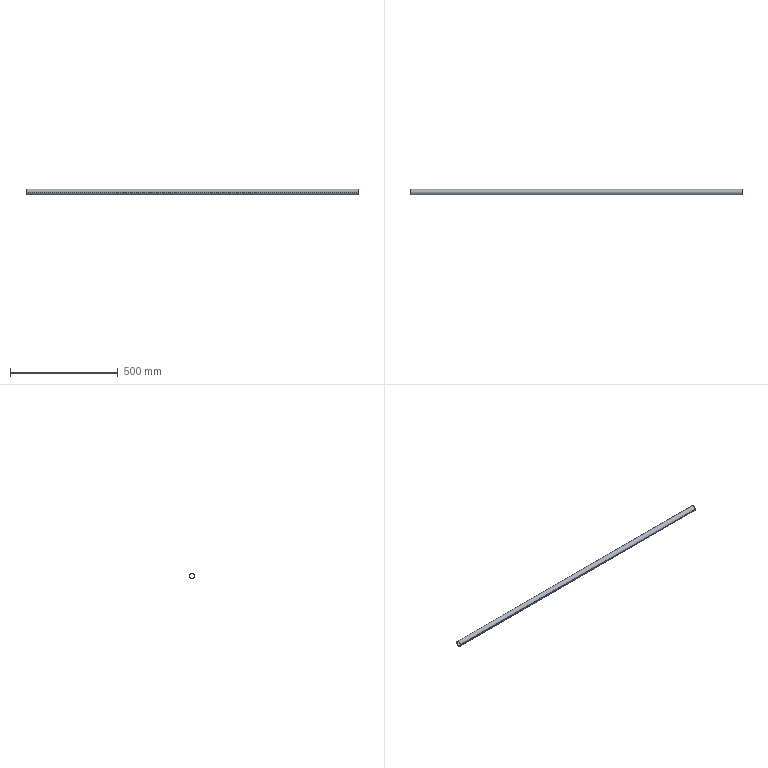Part | STEP file | E3-电柜护栏6栏杆_Default<As Machined> | 1 solid | 6 faces | box 1540 x 25 x 25 mm | volume 170541 mm3 | cylinder 4 | plane 2 | commonest cylinder face diameters 22 x2 25 x2
STEP:
#1=CARTESIAN_POINT('',(0.,0.,0.));
#2=DIRECTION('',(0.,0.,1.));
#3=DIRECTION('',(1.,0.,0.));
#4=AXIS2_PLACEMENT_3D('',#1,#2,#3);
#5=CARTESIAN_POINT('',(770.,-12.5,0.));
#6=VERTEX_POINT('',#5);
#7=CARTESIAN_POINT('',(770.,12.5,0.));
#8=VERTEX_POINT('',#7);
#9=CARTESIAN_POINT('',(770.,0.,0.));
#10=DIRECTION('',(-1.,0.,0.));
#11=DIRECTION('',(0.,1.,0.));
#12=AXIS2_PLACEMENT_3D('',#9,#10,#11);
#13=CIRCLE('',#12,12.5);
#14=CARTESIAN_POINT('',(770.,0.,0.));
#15=DIRECTION('',(-1.,0.,0.));
#16=DIRECTION('',(0.,-1.,0.));
#17=AXIS2_PLACEMENT_3D('',#14,#15,#16);
#18=CYLINDRICAL_SURFACE('',#17,12.5);
#19=CARTESIAN_POINT('',(-3.142,0.));
#20=DIRECTION('',(1.,0.));
#21=VECTOR('',#20,1.);
#22=LINE('',#19,#21);
#23=(GEOMETRIC_REPRESENTATION_CONTEXT(2)PARAMETRIC_REPRESENTATION_CONTEXT()REPRESENTATION_CONTEXT('',''));
#24=DEFINITIONAL_REPRESENTATION('',(#22),#23);
#25=PCURVE('',#18,#24);
#26=CARTESIAN_POINT('',(770.,0.,0.));
#27=DIRECTION('',(1.,0.,0.));
#28=DIRECTION('',(0.,1.,0.));
#29=AXIS2_PLACEMENT_3D('',#26,#27,#28);
#30=PLANE('',#29);
#31=CARTESIAN_POINT('',(12.5,0.));
#32=CARTESIAN_POINT('',(12.5,-21.651));
#33=CARTESIAN_POINT('',(-6.25,-10.825));
#34=CARTESIAN_POINT('',(-25.,0.));
#35=CARTESIAN_POINT('',(-6.25,10.825));
#36=CARTESIAN_POINT('',(12.5,21.651));
#37=CARTESIAN_POINT('',(12.5,0.));
#38=(BOUNDED_CURVE()B_SPLINE_CURVE(2,(#31,#32,#33,#34,#35,#36,#37),.UNSPECIFIED.,.T.,.F.)B_SPLINE_CURVE_WITH_KNOTS((1,2,2,2,2,1),(-2.094,0.,2.094,4.189,6.283,8.378),.UNSPECIFIED.)CURVE()GEOMETRIC_REPRESENTATION_ITEM()RATIONAL_B_SPLINE_CURVE((1.,0.5,1.,0.5,1.,0.5,1.))REPRESENTATION_ITEM(''));
#39=(GEOMETRIC_REPRESENTATION_CONTEXT(2)PARAMETRIC_REPRESENTATION_CONTEXT()REPRESENTATION_CONTEXT('',''));
#40=DEFINITIONAL_REPRESENTATION('',(#38),#39);
#41=PCURVE('',#30,#40);
#42=SURFACE_CURVE('',#13,(#25,#41),.PCURVE_S1.);
#43=EDGE_CURVE('',#6,#8,#42,.T.);
#44=ORIENTED_EDGE('',*,*,#43,.T.);
#45=CARTESIAN_POINT('',(-770.,12.5,0.));
#46=VERTEX_POINT('',#45);
#47=CARTESIAN_POINT('',(770.,12.5,0.));
#48=DIRECTION('',(-1.,0.,0.));
#49=VECTOR('',#48,1.);
#50=LINE('',#47,#49);
#51=CARTESIAN_POINT('',(3.142,0.));
#52=DIRECTION('',(0.,1.));
#53=VECTOR('',#52,1.);
#54=LINE('',#51,#53);
#55=(GEOMETRIC_REPRESENTATION_CONTEXT(2)PARAMETRIC_REPRESENTATION_CONTEXT()REPRESENTATION_CONTEXT('',''));
#56=DEFINITIONAL_REPRESENTATION('',(#54),#55);
#57=PCURVE('',#18,#56);
#58=CARTESIAN_POINT('',(770.,0.,0.));
#59=DIRECTION('',(-1.,0.,0.));
#60=DIRECTION('',(0.,-1.,0.));
#61=AXIS2_PLACEMENT_3D('',#58,#59,#60);
#62=CYLINDRICAL_SURFACE('',#61,12.5);
#63=CARTESIAN_POINT('',(3.142,0.));
#64=DIRECTION('',(0.,1.));
#65=VECTOR('',#64,1.);
#66=LINE('',#63,#65);
#67=(GEOMETRIC_REPRESENTATION_CONTEXT(2)PARAMETRIC_REPRESENTATION_CONTEXT()REPRESENTATION_CONTEXT('',''));
#68=DEFINITIONAL_REPRESENTATION('',(#66),#67);
#69=PCURVE('',#62,#68);
#70=SURFACE_CURVE('',#50,(#57,#69),.PCURVE_S1.);
#71=EDGE_CURVE('',#8,#46,#70,.T.);
#72=ORIENTED_EDGE('',*,*,#71,.T.);
#73=CARTESIAN_POINT('',(-770.,-12.5,0.));
#74=VERTEX_POINT('',#73);
#75=CARTESIAN_POINT('',(-770.,0.,0.));
#76=DIRECTION('',(-1.,0.,0.));
#77=DIRECTION('',(0.,1.,0.));
#78=AXIS2_PLACEMENT_3D('',#75,#76,#77);
#79=CIRCLE('',#78,12.5);
#80=CARTESIAN_POINT('',(-3.142,1540.));
#81=DIRECTION('',(1.,0.));
#82=VECTOR('',#81,1.);
#83=LINE('',#80,#82);
#84=(GEOMETRIC_REPRESENTATION_CONTEXT(2)PARAMETRIC_REPRESENTATION_CONTEXT()REPRESENTATION_CONTEXT('',''));
#85=DEFINITIONAL_REPRESENTATION('',(#83),#84);
#86=PCURVE('',#18,#85);
#87=CARTESIAN_POINT('',(-770.,0.,0.));
#88=DIRECTION('',(1.,0.,0.));
#89=DIRECTION('',(0.,1.,0.));
#90=AXIS2_PLACEMENT_3D('',#87,#88,#89);
#91=PLANE('',#90);
#92=CARTESIAN_POINT('',(12.5,0.));
#93=CARTESIAN_POINT('',(12.5,-21.651));
#94=CARTESIAN_POINT('',(-6.25,-10.825));
#95=CARTESIAN_POINT('',(-25.,0.));
#96=CARTESIAN_POINT('',(-6.25,10.825));
#97=CARTESIAN_POINT('',(12.5,21.651));
#98=CARTESIAN_POINT('',(12.5,0.));
#99=(BOUNDED_CURVE()B_SPLINE_CURVE(2,(#92,#93,#94,#95,#96,#97,#98),.UNSPECIFIED.,.T.,.F.)B_SPLINE_CURVE_WITH_KNOTS((1,2,2,2,2,1),(-2.094,0.,2.094,4.189,6.283,8.378),.UNSPECIFIED.)CURVE()GEOMETRIC_REPRESENTATION_ITEM()RATIONAL_B_SPLINE_CURVE((1.,0.5,1.,0.5,1.,0.5,1.))REPRESENTATION_ITEM(''));
#100=(GEOMETRIC_REPRESENTATION_CONTEXT(2)PARAMETRIC_REPRESENTATION_CONTEXT()REPRESENTATION_CONTEXT('',''));
#101=DEFINITIONAL_REPRESENTATION('',(#99),#100);
#102=PCURVE('',#91,#101);
#103=SURFACE_CURVE('',#79,(#86,#102),.PCURVE_S1.);
#104=EDGE_CURVE('',#74,#46,#103,.T.);
#105=ORIENTED_EDGE('',*,*,#104,.F.);
#106=CARTESIAN_POINT('',(770.,-12.5,0.));
#107=DIRECTION('',(-1.,0.,0.));
#108=VECTOR('',#107,1.);
#109=LINE('',#106,#108);
#110=CARTESIAN_POINT('',(0.,0.));
#111=DIRECTION('',(0.,1.));
#112=VECTOR('',#111,1.);
#113=LINE('',#110,#112);
#114=(GEOMETRIC_REPRESENTATION_CONTEXT(2)PARAMETRIC_REPRESENTATION_CONTEXT()REPRESENTATION_CONTEXT('',''));
#115=DEFINITIONAL_REPRESENTATION('',(#113),#114);
#116=PCURVE('',#18,#115);
#117=CARTESIAN_POINT('',(6.283,0.));
#118=DIRECTION('',(0.,1.));
#119=VECTOR('',#118,1.);
#120=LINE('',#117,#119);
#121=(GEOMETRIC_REPRESENTATION_CONTEXT(2)PARAMETRIC_REPRESENTATION_CONTEXT()REPRESENTATION_CONTEXT('',''));
#122=DEFINITIONAL_REPRESENTATION('',(#120),#121);
#123=PCURVE('',#62,#122);
#124=SURFACE_CURVE('',#109,(#116,#123),.PCURVE_S1.);
#125=EDGE_CURVE('',#6,#74,#124,.T.);
#126=ORIENTED_EDGE('',*,*,#125,.F.);
#127=EDGE_LOOP('',(#44,#72,#105,#126));
#128=FACE_BOUND('',#127,.T.);
#129=ADVANCED_FACE('',(#128),#18,.T.);
#130=CARTESIAN_POINT('',(770.,-11.,0.));
#131=VERTEX_POINT('',#130);
#132=CARTESIAN_POINT('',(-770.,-11.,0.));
#133=VERTEX_POINT('',#132);
#134=CARTESIAN_POINT('',(770.,-11.,0.));
#135=DIRECTION('',(-1.,0.,0.));
#136=VECTOR('',#135,1.);
#137=LINE('',#134,#136);
#138=CARTESIAN_POINT('',(770.,0.,0.));
#139=DIRECTION('',(-1.,0.,0.));
#140=DIRECTION('',(0.,-1.,0.));
#141=AXIS2_PLACEMENT_3D('',#138,#139,#140);
#142=CYLINDRICAL_SURFACE('',#141,11.);
#143=CARTESIAN_POINT('',(6.283,0.));
#144=DIRECTION('',(0.,1.));
#145=VECTOR('',#144,1.);
#146=LINE('',#143,#145);
#147=(GEOMETRIC_REPRESENTATION_CONTEXT(2)PARAMETRIC_REPRESENTATION_CONTEXT()REPRESENTATION_CONTEXT('',''));
#148=DEFINITIONAL_REPRESENTATION('',(#146),#147);
#149=PCURVE('',#142,#148);
#150=CARTESIAN_POINT('',(770.,0.,0.));
#151=DIRECTION('',(-1.,0.,0.));
#152=DIRECTION('',(0.,-1.,0.));
#153=AXIS2_PLACEMENT_3D('',#150,#151,#152);
#154=CYLINDRICAL_SURFACE('',#153,11.);
#155=CARTESIAN_POINT('',(0.,0.));
#156=DIRECTION('',(0.,1.));
#157=VECTOR('',#156,1.);
#158=LINE('',#155,#157);
#159=(GEOMETRIC_REPRESENTATION_CONTEXT(2)PARAMETRIC_REPRESENTATION_CONTEXT()REPRESENTATION_CONTEXT('',''));
#160=DEFINITIONAL_REPRESENTATION('',(#158),#159);
#161=PCURVE('',#154,#160);
#162=SURFACE_CURVE('',#137,(#149,#161),.PCURVE_S1.);
#163=EDGE_CURVE('',#131,#133,#162,.T.);
#164=ORIENTED_EDGE('',*,*,#163,.T.);
#165=CARTESIAN_POINT('',(-770.,11.,0.));
#166=VERTEX_POINT('',#165);
#167=CARTESIAN_POINT('',(-770.,0.,0.));
#168=DIRECTION('',(-1.,0.,0.));
#169=DIRECTION('',(0.,1.,0.));
#170=AXIS2_PLACEMENT_3D('',#167,#168,#169);
#171=CIRCLE('',#170,11.);
#172=CARTESIAN_POINT('',(3.142,1540.));
#173=DIRECTION('',(1.,0.));
#174=VECTOR('',#173,1.);
#175=LINE('',#172,#174);
#176=(GEOMETRIC_REPRESENTATION_CONTEXT(2)PARAMETRIC_REPRESENTATION_CONTEXT()REPRESENTATION_CONTEXT('',''));
#177=DEFINITIONAL_REPRESENTATION('',(#175),#176);
#178=PCURVE('',#142,#177);
#179=CARTESIAN_POINT('',(11.,0.));
#180=CARTESIAN_POINT('',(11.,-19.053));
#181=CARTESIAN_POINT('',(-5.5,-9.526));
#182=CARTESIAN_POINT('',(-22.,0.));
#183=CARTESIAN_POINT('',(-5.5,9.526));
#184=CARTESIAN_POINT('',(11.,19.053));
#185=CARTESIAN_POINT('',(11.,0.));
#186=(BOUNDED_CURVE()B_SPLINE_CURVE(2,(#179,#180,#181,#182,#183,#184,#185),.UNSPECIFIED.,.T.,.F.)B_SPLINE_CURVE_WITH_KNOTS((1,2,2,2,2,1),(-2.094,0.,2.094,4.189,6.283,8.378),.UNSPECIFIED.)CURVE()GEOMETRIC_REPRESENTATION_ITEM()RATIONAL_B_SPLINE_CURVE((1.,0.5,1.,0.5,1.,0.5,1.))REPRESENTATION_ITEM(''));
#187=(GEOMETRIC_REPRESENTATION_CONTEXT(2)PARAMETRIC_REPRESENTATION_CONTEXT()REPRESENTATION_CONTEXT('',''));
#188=DEFINITIONAL_REPRESENTATION('',(#186),#187);
#189=PCURVE('',#91,#188);
#190=SURFACE_CURVE('',#171,(#178,#189),.PCURVE_S1.);
#191=EDGE_CURVE('',#166,#133,#190,.T.);
#192=ORIENTED_EDGE('',*,*,#191,.F.);
#193=CARTESIAN_POINT('',(770.,11.,0.));
#194=VERTEX_POINT('',#193);
#195=CARTESIAN_POINT('',(770.,11.,0.));
#196=DIRECTION('',(-1.,0.,0.));
#197=VECTOR('',#196,1.);
#198=LINE('',#195,#197);
#199=CARTESIAN_POINT('',(3.142,0.));
#200=DIRECTION('',(0.,1.));
#201=VECTOR('',#200,1.);
#202=LINE('',#199,#201);
#203=(GEOMETRIC_REPRESENTATION_CONTEXT(2)PARAMETRIC_REPRESENTATION_CONTEXT()REPRESENTATION_CONTEXT('',''));
#204=DEFINITIONAL_REPRESENTATION('',(#202),#203);
#205=PCURVE('',#142,#204);
#206=CARTESIAN_POINT('',(3.142,0.));
#207=DIRECTION('',(0.,1.));
#208=VECTOR('',#207,1.);
#209=LINE('',#206,#208);
#210=(GEOMETRIC_REPRESENTATION_CONTEXT(2)PARAMETRIC_REPRESENTATION_CONTEXT()REPRESENTATION_CONTEXT('',''));
#211=DEFINITIONAL_REPRESENTATION('',(#209),#210);
#212=PCURVE('',#154,#211);
#213=SURFACE_CURVE('',#198,(#205,#212),.PCURVE_S1.);
#214=EDGE_CURVE('',#194,#166,#213,.T.);
#215=ORIENTED_EDGE('',*,*,#214,.F.);
#216=CARTESIAN_POINT('',(770.,0.,0.));
#217=DIRECTION('',(-1.,0.,0.));
#218=DIRECTION('',(0.,1.,0.));
#219=AXIS2_PLACEMENT_3D('',#216,#217,#218);
#220=CIRCLE('',#219,11.);
#221=CARTESIAN_POINT('',(3.142,0.));
#222=DIRECTION('',(1.,0.));
#223=VECTOR('',#222,1.);
#224=LINE('',#221,#223);
#225=(GEOMETRIC_REPRESENTATION_CONTEXT(2)PARAMETRIC_REPRESENTATION_CONTEXT()REPRESENTATION_CONTEXT('',''));
#226=DEFINITIONAL_REPRESENTATION('',(#224),#225);
#227=PCURVE('',#142,#226);
#228=CARTESIAN_POINT('',(11.,0.));
#229=CARTESIAN_POINT('',(11.,-19.053));
#230=CARTESIAN_POINT('',(-5.5,-9.526));
#231=CARTESIAN_POINT('',(-22.,0.));
#232=CARTESIAN_POINT('',(-5.5,9.526));
#233=CARTESIAN_POINT('',(11.,19.053));
#234=CARTESIAN_POINT('',(11.,0.));
#235=(BOUNDED_CURVE()B_SPLINE_CURVE(2,(#228,#229,#230,#231,#232,#233,#234),.UNSPECIFIED.,.T.,.F.)B_SPLINE_CURVE_WITH_KNOTS((1,2,2,2,2,1),(-2.094,0.,2.094,4.189,6.283,8.378),.UNSPECIFIED.)CURVE()GEOMETRIC_REPRESENTATION_ITEM()RATIONAL_B_SPLINE_CURVE((1.,0.5,1.,0.5,1.,0.5,1.))REPRESENTATION_ITEM(''));
#236=(GEOMETRIC_REPRESENTATION_CONTEXT(2)PARAMETRIC_REPRESENTATION_CONTEXT()REPRESENTATION_CONTEXT('',''));
#237=DEFINITIONAL_REPRESENTATION('',(#235),#236);
#238=PCURVE('',#30,#237);
#239=SURFACE_CURVE('',#220,(#227,#238),.PCURVE_S1.);
#240=EDGE_CURVE('',#194,#131,#239,.T.);
#241=ORIENTED_EDGE('',*,*,#240,.T.);
#242=EDGE_LOOP('',(#164,#192,#215,#241));
#243=FACE_BOUND('',#242,.F.);
#244=ADVANCED_FACE('',(#243),#142,.F.);
#245=CARTESIAN_POINT('',(-770.,0.,0.));
#246=DIRECTION('',(-1.,0.,0.));
#247=DIRECTION('',(0.,1.,0.));
#248=AXIS2_PLACEMENT_3D('',#245,#246,#247);
#249=CIRCLE('',#248,11.);
#250=CARTESIAN_POINT('',(-3.142,1540.));
#251=DIRECTION('',(1.,0.));
#252=VECTOR('',#251,1.);
#253=LINE('',#250,#252);
#254=(GEOMETRIC_REPRESENTATION_CONTEXT(2)PARAMETRIC_REPRESENTATION_CONTEXT()REPRESENTATION_CONTEXT('',''));
#255=DEFINITIONAL_REPRESENTATION('',(#253),#254);
#256=PCURVE('',#154,#255);
#257=CARTESIAN_POINT('',(11.,0.));
#258=CARTESIAN_POINT('',(11.,-19.053));
#259=CARTESIAN_POINT('',(-5.5,-9.526));
#260=CARTESIAN_POINT('',(-22.,0.));
#261=CARTESIAN_POINT('',(-5.5,9.526));
#262=CARTESIAN_POINT('',(11.,19.053));
#263=CARTESIAN_POINT('',(11.,0.));
#264=(BOUNDED_CURVE()B_SPLINE_CURVE(2,(#257,#258,#259,#260,#261,#262,#263),.UNSPECIFIED.,.T.,.F.)B_SPLINE_CURVE_WITH_KNOTS((1,2,2,2,2,1),(-2.094,0.,2.094,4.189,6.283,8.378),.UNSPECIFIED.)CURVE()GEOMETRIC_REPRESENTATION_ITEM()RATIONAL_B_SPLINE_CURVE((1.,0.5,1.,0.5,1.,0.5,1.))REPRESENTATION_ITEM(''));
#265=(GEOMETRIC_REPRESENTATION_CONTEXT(2)PARAMETRIC_REPRESENTATION_CONTEXT()REPRESENTATION_CONTEXT('',''));
#266=DEFINITIONAL_REPRESENTATION('',(#264),#265);
#267=PCURVE('',#91,#266);
#268=SURFACE_CURVE('',#249,(#256,#267),.PCURVE_S1.);
#269=EDGE_CURVE('',#133,#166,#268,.T.);
#270=ORIENTED_EDGE('',*,*,#269,.F.);
#271=ORIENTED_EDGE('',*,*,#163,.F.);
#272=CARTESIAN_POINT('',(770.,0.,0.));
#273=DIRECTION('',(-1.,0.,0.));
#274=DIRECTION('',(0.,1.,0.));
#275=AXIS2_PLACEMENT_3D('',#272,#273,#274);
#276=CIRCLE('',#275,11.);
#277=CARTESIAN_POINT('',(-3.142,0.));
#278=DIRECTION('',(1.,0.));
#279=VECTOR('',#278,1.);
#280=LINE('',#277,#279);
#281=(GEOMETRIC_REPRESENTATION_CONTEXT(2)PARAMETRIC_REPRESENTATION_CONTEXT()REPRESENTATION_CONTEXT('',''));
#282=DEFINITIONAL_REPRESENTATION('',(#280),#281);
#283=PCURVE('',#154,#282);
#284=CARTESIAN_POINT('',(11.,0.));
#285=CARTESIAN_POINT('',(11.,-19.053));
#286=CARTESIAN_POINT('',(-5.5,-9.526));
#287=CARTESIAN_POINT('',(-22.,0.));
#288=CARTESIAN_POINT('',(-5.5,9.526));
#289=CARTESIAN_POINT('',(11.,19.053));
#290=CARTESIAN_POINT('',(11.,0.));
#291=(BOUNDED_CURVE()B_SPLINE_CURVE(2,(#284,#285,#286,#287,#288,#289,#290),.UNSPECIFIED.,.T.,.F.)B_SPLINE_CURVE_WITH_KNOTS((1,2,2,2,2,1),(-2.094,0.,2.094,4.189,6.283,8.378),.UNSPECIFIED.)CURVE()GEOMETRIC_REPRESENTATION_ITEM()RATIONAL_B_SPLINE_CURVE((1.,0.5,1.,0.5,1.,0.5,1.))REPRESENTATION_ITEM(''));
#292=(GEOMETRIC_REPRESENTATION_CONTEXT(2)PARAMETRIC_REPRESENTATION_CONTEXT()REPRESENTATION_CONTEXT('',''));
#293=DEFINITIONAL_REPRESENTATION('',(#291),#292);
#294=PCURVE('',#30,#293);
#295=SURFACE_CURVE('',#276,(#283,#294),.PCURVE_S1.);
#296=EDGE_CURVE('',#131,#194,#295,.T.);
#297=ORIENTED_EDGE('',*,*,#296,.T.);
#298=ORIENTED_EDGE('',*,*,#214,.T.);
#299=EDGE_LOOP('',(#270,#271,#297,#298));
#300=FACE_BOUND('',#299,.F.);
#301=ADVANCED_FACE('',(#300),#154,.F.);
#302=ORIENTED_EDGE('',*,*,#71,.F.);
#303=CARTESIAN_POINT('',(770.,0.,0.));
#304=DIRECTION('',(-1.,0.,0.));
#305=DIRECTION('',(0.,1.,0.));
#306=AXIS2_PLACEMENT_3D('',#303,#304,#305);
#307=CIRCLE('',#306,12.5);
#308=CARTESIAN_POINT('',(3.142,0.));
#309=DIRECTION('',(1.,0.));
#310=VECTOR('',#309,1.);
#311=LINE('',#308,#310);
#312=(GEOMETRIC_REPRESENTATION_CONTEXT(2)PARAMETRIC_REPRESENTATION_CONTEXT()REPRESENTATION_CONTEXT('',''));
#313=DEFINITIONAL_REPRESENTATION('',(#311),#312);
#314=PCURVE('',#62,#313);
#315=CARTESIAN_POINT('',(12.5,0.));
#316=CARTESIAN_POINT('',(12.5,-21.651));
#317=CARTESIAN_POINT('',(-6.25,-10.825));
#318=CARTESIAN_POINT('',(-25.,0.));
#319=CARTESIAN_POINT('',(-6.25,10.825));
#320=CARTESIAN_POINT('',(12.5,21.651));
#321=CARTESIAN_POINT('',(12.5,0.));
#322=(BOUNDED_CURVE()B_SPLINE_CURVE(2,(#315,#316,#317,#318,#319,#320,#321),.UNSPECIFIED.,.T.,.F.)B_SPLINE_CURVE_WITH_KNOTS((1,2,2,2,2,1),(-2.094,0.,2.094,4.189,6.283,8.378),.UNSPECIFIED.)CURVE()GEOMETRIC_REPRESENTATION_ITEM()RATIONAL_B_SPLINE_CURVE((1.,0.5,1.,0.5,1.,0.5,1.))REPRESENTATION_ITEM(''));
#323=(GEOMETRIC_REPRESENTATION_CONTEXT(2)PARAMETRIC_REPRESENTATION_CONTEXT()REPRESENTATION_CONTEXT('',''));
#324=DEFINITIONAL_REPRESENTATION('',(#322),#323);
#325=PCURVE('',#30,#324);
#326=SURFACE_CURVE('',#307,(#314,#325),.PCURVE_S1.);
#327=EDGE_CURVE('',#8,#6,#326,.T.);
#328=ORIENTED_EDGE('',*,*,#327,.T.);
#329=ORIENTED_EDGE('',*,*,#125,.T.);
#330=CARTESIAN_POINT('',(-770.,0.,0.));
#331=DIRECTION('',(-1.,0.,0.));
#332=DIRECTION('',(0.,1.,0.));
#333=AXIS2_PLACEMENT_3D('',#330,#331,#332);
#334=CIRCLE('',#333,12.5);
#335=CARTESIAN_POINT('',(3.142,1540.));
#336=DIRECTION('',(1.,0.));
#337=VECTOR('',#336,1.);
#338=LINE('',#335,#337);
#339=(GEOMETRIC_REPRESENTATION_CONTEXT(2)PARAMETRIC_REPRESENTATION_CONTEXT()REPRESENTATION_CONTEXT('',''));
#340=DEFINITIONAL_REPRESENTATION('',(#338),#339);
#341=PCURVE('',#62,#340);
#342=CARTESIAN_POINT('',(12.5,0.));
#343=CARTESIAN_POINT('',(12.5,-21.651));
#344=CARTESIAN_POINT('',(-6.25,-10.825));
#345=CARTESIAN_POINT('',(-25.,0.));
#346=CARTESIAN_POINT('',(-6.25,10.825));
#347=CARTESIAN_POINT('',(12.5,21.651));
#348=CARTESIAN_POINT('',(12.5,0.));
#349=(BOUNDED_CURVE()B_SPLINE_CURVE(2,(#342,#343,#344,#345,#346,#347,#348),.UNSPECIFIED.,.T.,.F.)B_SPLINE_CURVE_WITH_KNOTS((1,2,2,2,2,1),(-2.094,0.,2.094,4.189,6.283,8.378),.UNSPECIFIED.)CURVE()GEOMETRIC_REPRESENTATION_ITEM()RATIONAL_B_SPLINE_CURVE((1.,0.5,1.,0.5,1.,0.5,1.))REPRESENTATION_ITEM(''));
#350=(GEOMETRIC_REPRESENTATION_CONTEXT(2)PARAMETRIC_REPRESENTATION_CONTEXT()REPRESENTATION_CONTEXT('',''));
#351=DEFINITIONAL_REPRESENTATION('',(#349),#350);
#352=PCURVE('',#91,#351);
#353=SURFACE_CURVE('',#334,(#341,#352),.PCURVE_S1.);
#354=EDGE_CURVE('',#46,#74,#353,.T.);
#355=ORIENTED_EDGE('',*,*,#354,.F.);
#356=EDGE_LOOP('',(#302,#328,#329,#355));
#357=FACE_BOUND('',#356,.T.);
#358=ADVANCED_FACE('',(#357),#62,.T.);
#359=ORIENTED_EDGE('',*,*,#296,.T.);
#360=ORIENTED_EDGE('',*,*,#240,.T.);
#361=EDGE_LOOP('',(#359,#360));
#362=FACE_BOUND('',#361,.T.);
#363=ORIENTED_EDGE('',*,*,#43,.F.);
#364=ORIENTED_EDGE('',*,*,#327,.F.);
#365=EDGE_LOOP('',(#363,#364));
#366=FACE_BOUND('',#365,.T.);
#367=ADVANCED_FACE('',(#362,#366),#30,.T.);
#368=ORIENTED_EDGE('',*,*,#269,.F.);
#369=ORIENTED_EDGE('',*,*,#191,.F.);
#370=EDGE_LOOP('',(#368,#369));
#371=FACE_BOUND('',#370,.T.);
#372=ORIENTED_EDGE('',*,*,#104,.T.);
#373=ORIENTED_EDGE('',*,*,#354,.T.);
#374=EDGE_LOOP('',(#372,#373));
#375=FACE_BOUND('',#374,.T.);
#376=ADVANCED_FACE('',(#371,#375),#91,.F.);
#377=CLOSED_SHELL('',(#129,#244,#301,#358,#367,#376));
#378=MANIFOLD_SOLID_BREP('',#377);
#379=(LENGTH_UNIT()NAMED_UNIT(*)SI_UNIT(.MILLI.,.METRE.));
#380=UNCERTAINTY_MEASURE_WITH_UNIT(LENGTH_MEASURE(0.0000001),#379,'','');
#381=(NAMED_UNIT(*)PLANE_ANGLE_UNIT()SI_UNIT($,.RADIAN.));
#382=(NAMED_UNIT(*)SI_UNIT($,.STERADIAN.)SOLID_ANGLE_UNIT());
#383=(GEOMETRIC_REPRESENTATION_CONTEXT(3)GLOBAL_UNCERTAINTY_ASSIGNED_CONTEXT((#380))GLOBAL_UNIT_ASSIGNED_CONTEXT((#379,#381,#382))REPRESENTATION_CONTEXT('',''));
#384=ADVANCED_BREP_SHAPE_REPRESENTATION('',(#4,#378),#383);